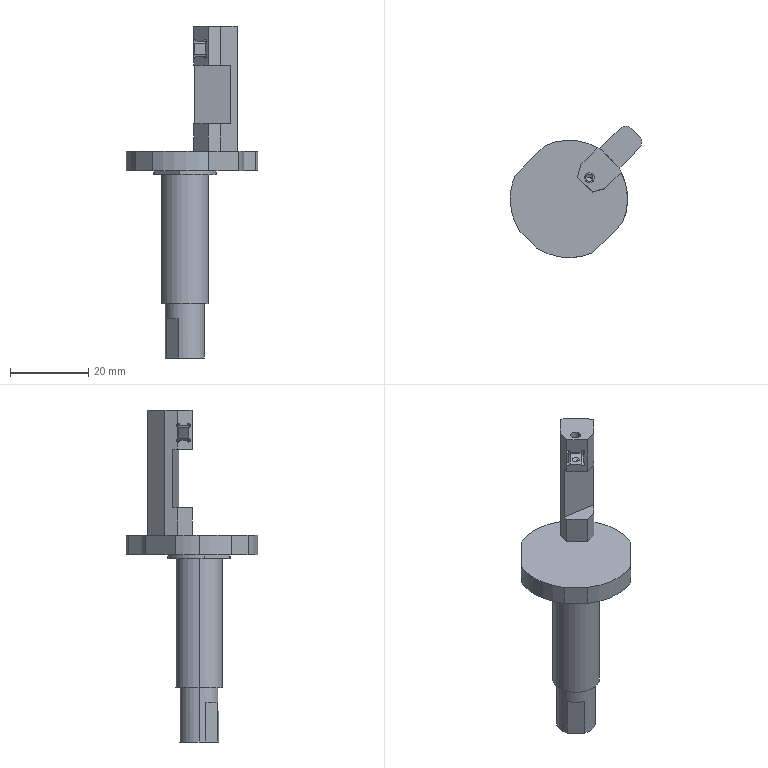Part | STEP file | 04-02 bending swing lever | 1 solid | 63 faces | box 33.617 x 33.617 x 84.85 mm | volume 10597 mm3 | plane 36 | cylinder 25 | cone 2 | commonest cylinder face diameters 1 x6 30 x5 2.5 x4 4 x3 16 x3 10 x2